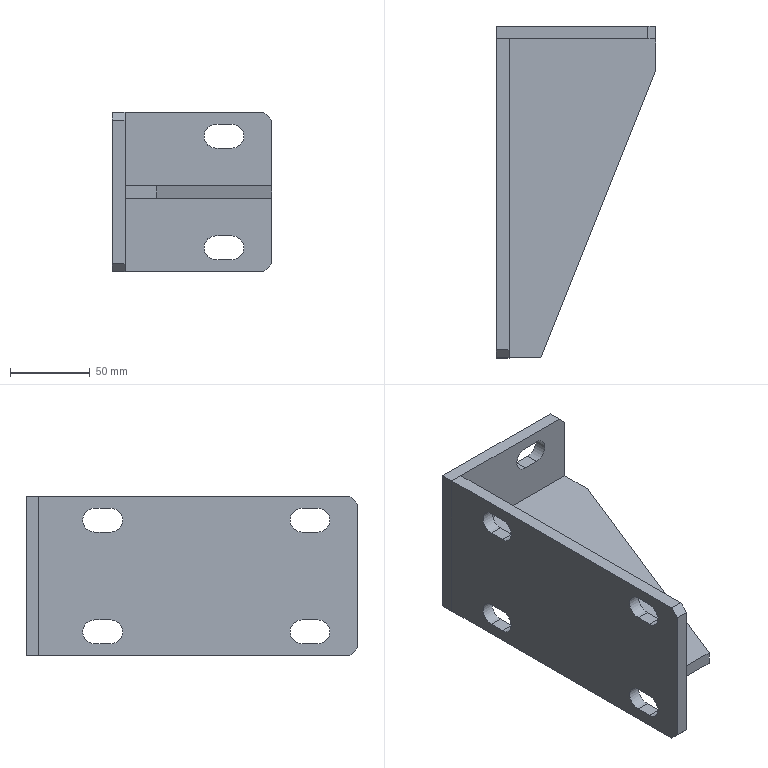Part | STEP file | E3-Diagonal plate 100-1 | 2 solids | 45 faces | box 100 x 208 x 100 mm | volume 319278 mm3 | plane 33 | cylinder 12 | commonest cylinder face diameters 15 x12